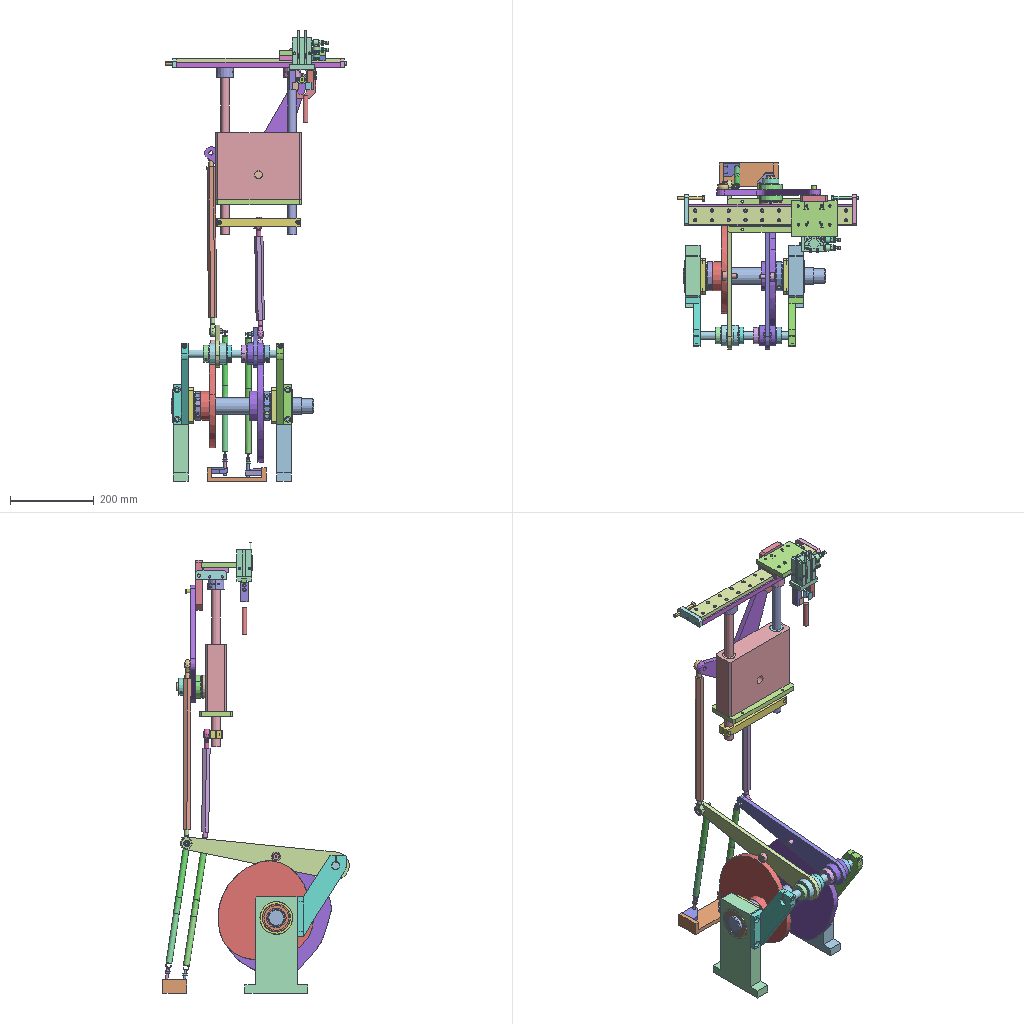Assembly | NX | 112 different items | 112 placed | box 434 x 445 x 1076 mm
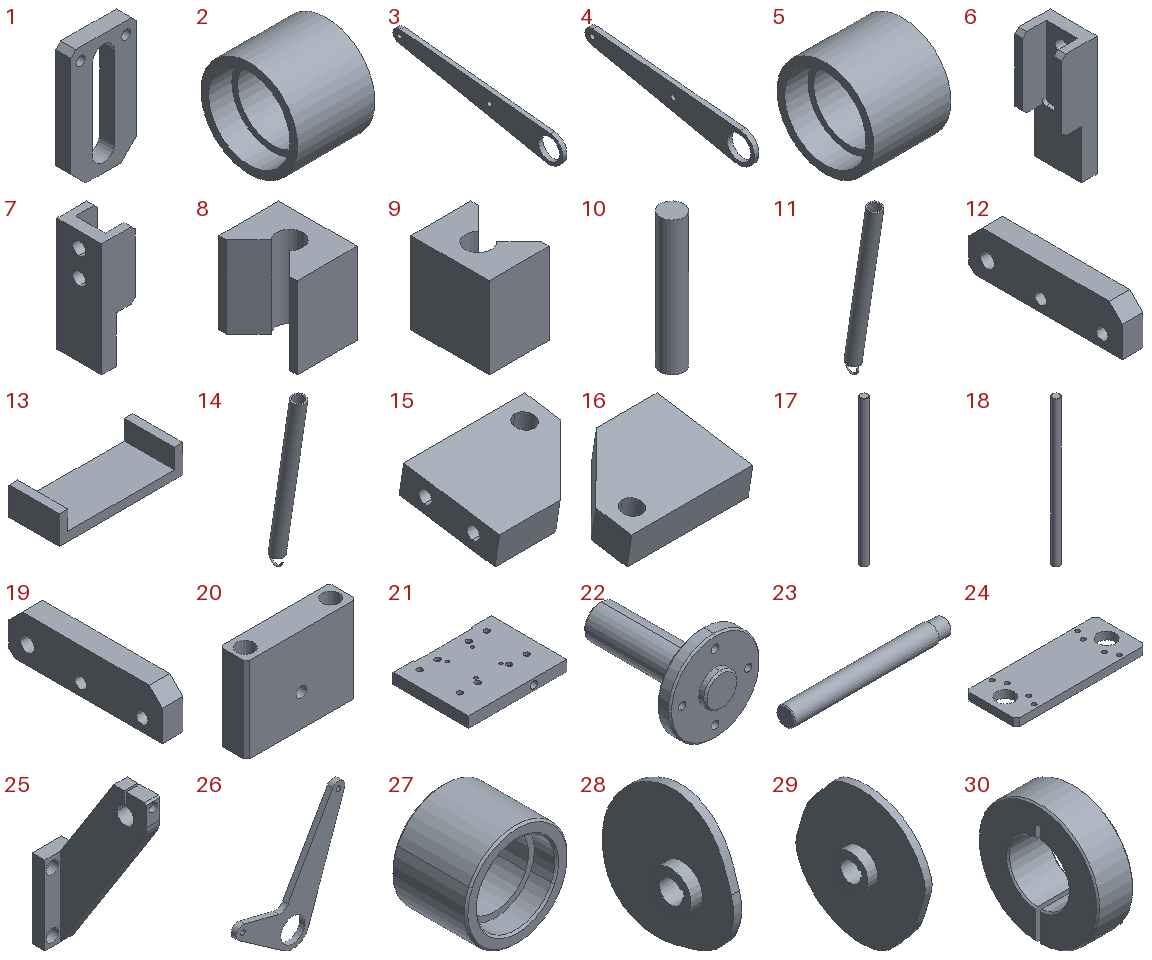Parts list (item | quantity | size | volume | features):
1 | x1 | 65 x 15 x 120 mm | 77204 mm3 | features 001 2
2 | x1 | 40 x 50 x 50 mm | 29003 mm3 | features _-17204000 2
3 | x1 | 10 x 403.429 x 100.813 mm | 170075 mm3 | features _-17232000 2
4 | x1 | 10 x 359.893 x 95.107 mm | 149250 mm3 | features _-17372000 2
5 | x1 | 40 x 50 x 50 mm | 29003 mm3 | features _-17667000 2
6 | x1 | 13.5 x 18 x 45.75 mm | 5474 mm3 | features 倒角2 2
7 | x1 | 13.5 x 18 x 45.75 mm | 5474 mm3 | features 倒角2 2
8 | x1 | 13.775 x 18 x 18.75 mm | 3258 mm3 | features solid 2
9 | x1 | 13.775 x 18 x 18.75 mm | 3258 mm3 | features solid 2
10 | x1 | 11 x 11 x 63 mm | 5987 mm3 | features solid 2
11 | x1 | 14 x 38.697 x 170.602 mm | 9414 mm3 | features solid 2
12 | x1 | 10 x 75 x 21.5 mm | 14819 mm3 | features 001 2
13 | x1 | 141.082 x 56.961 x 32.177 mm | 105625 mm3 | features solid 2
14 | x1 | 14 x 38.402 x 171.464 mm | 9463 mm3 | features solid 2
15 | x1 | 40 x 33.128 x 14.63 mm | 10189 mm3 | features 实体1 2
16 | x1 | 40 x 33.141 x 14.707 mm | 10189 mm3 | features 实体1 2
17 | x1 | 20 x 20 x 400 mm | 125603 mm3 | features 001 2
18 | x1 | 20 x 20 x 400 mm | 125603 mm3 | features 001 2
19 | x1 | 10 x 75 x 21.5 mm | 14819 mm3 | features 001 2
20 | x1 | 205 x 50 x 160 mm | 1357581 mm3 | features 001 2
21 | x1 | 110 x 85 x 12 mm | 106361 mm3 | features 00 2
22 | x1 | 55 x 74 x 55 mm | 38722 mm3 | features 00 2
23 | x1 | 340 x 40 x 40 mm | 417966 mm3 | features 00 2
24 | x1 | 205 x 80 x 12 mm | 176533 mm3 | features 00 2
25 | x1 | 35 x 116.8 x 193.095 mm | 171641 mm3 | features 0004 2
26 | x1 | 247.496 x 12 x 279.945 mm | 214925 mm3 | features 0 2
27 | x1 | 55 x 40 x 55 mm | 45192 mm3 | features 0 2
28 | x1 | 34 x 228.009 x 236.372 mm | 622668 mm3 | features 100X000 2
29 | x1 | 34 x 262.59 x 269.999 mm | 781015 mm3 | features 146X000 2
30 | x1 | 14 x 40 x 39.986 mm | 10434 mm3 | features 1_11 2
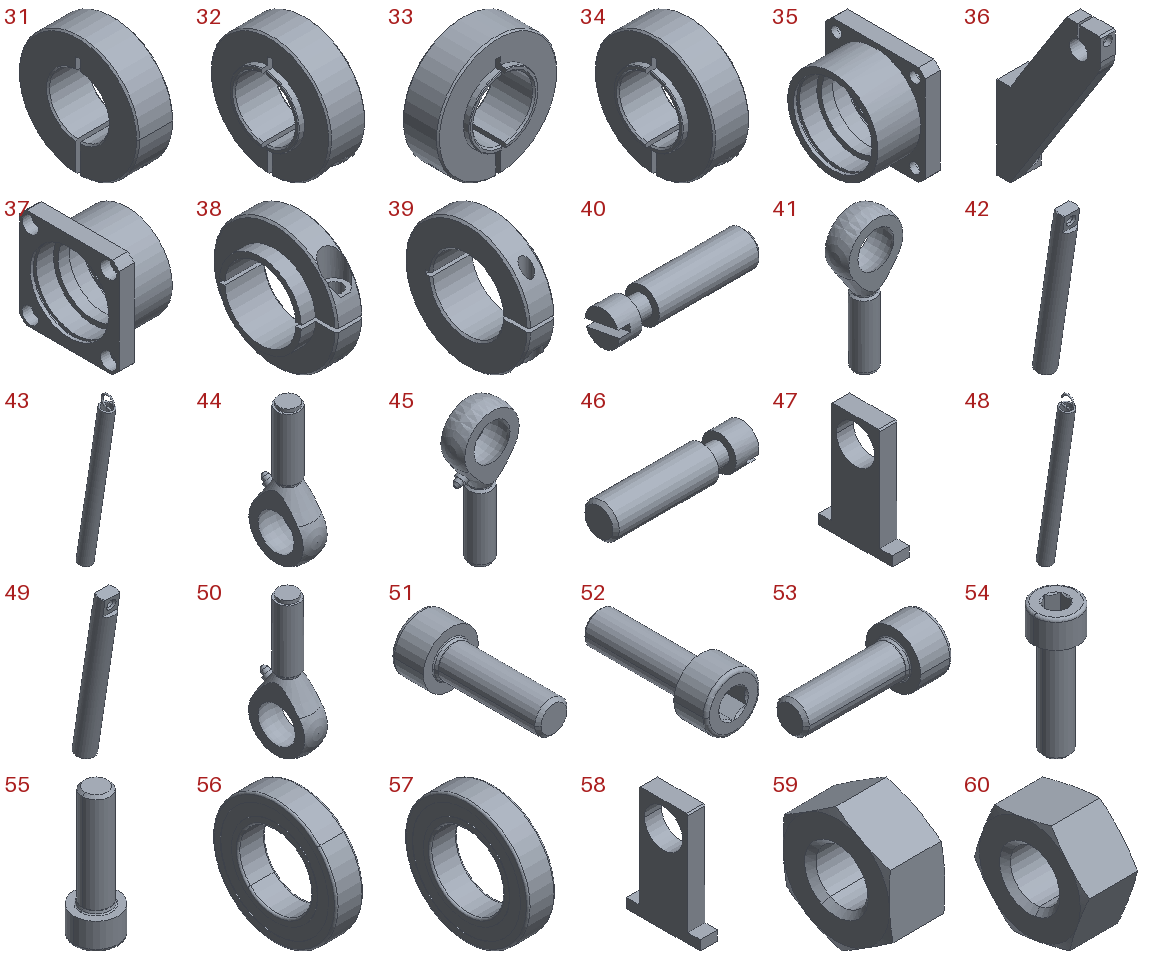31 | x1 | 14 x 40 x 39.986 mm | 10434 mm3 | features 1_11 2
32 | x1 | 14 x 40 x 39.986 mm | 10434 mm3 | features 1_11 2
33 | x1 | 40 x 14 x 39.986 mm | 10434 mm3 | features 1_11 2
34 | x1 | 14 x 40 x 39.986 mm | 10434 mm3 | features 1_11 2
35 | x1 | 50 x 86 x 86 mm | 89594 mm3 | features 1_1 2
36 | x1 | 35 x 116.8 x 193.095 mm | 171641 mm3 | features 0005 2
37 | x1 | 50 x 86 x 86 mm | 89594 mm3 | features 1_1 2
38 | x1 | 23 x 69.986 x 70 mm | 38156 mm3 | features 1_52 2
39 | x1 | 23 x 69.986 x 70 mm | 38156 mm3 | features 1_52 2
40 | x1 | 25 x 6 x 6 mm | 635.671 mm3 | features 1 2
41 | x1 | 26 x 10.639 x 61.044 mm | 5586 mm3 | features 1 2
42 | x1 | 6 x 12.52 x 50.075 mm | 1355 mm3 | features 1 2
43 | x1 | 14 x 39.013 x 172.675 mm | 9539 mm3 | features 1 2
44 | x1 | 11.237 x 26 x 61.087 mm | 5586 mm3 | features 1 2
45 | x1 | 26 x 11.258 x 61.087 mm | 5586 mm3 | features 1 2
46 | x1 | 25 x 6 x 6 mm | 635.671 mm3 | features 1 2
47 | x1 | 35 x 150 x 230 mm | 672442 mm3 | features 0006 2
48 | x1 | 14 x 38.473 x 171.94 mm | 9491 mm3 | features 1 2
49 | x1 | 6 x 12.629 x 50.067 mm | 1355 mm3 | features 1 2
50 | x1 | 11.496 x 26 x 61.044 mm | 5586 mm3 | features 1 2
51 | x1 | 8.5 x 21 x 8.5 mm | 547.645 mm3 | features 2_11 2
52 | x1 | 8.5 x 21 x 8.5 mm | 547.645 mm3 | features 2_11 2
53 | x1 | 21 x 8.5 x 8.5 mm | 547.645 mm3 | features 2_11 2
54 | x1 | 13 x 13 x 38 mm | 2398 mm3 | features 2_12 2
55 | x1 | 13 x 13 x 38 mm | 2398 mm3 | features 2_12 2
56 | x1 | 15 x 68 x 68 mm | 34781 mm3 | features 2_1 2
57 | x1 | 15 x 68 x 68 mm | 34781 mm3 | features 2_1 2
58 | x1 | 35 x 150 x 230 mm | 672442 mm3 | features 0006 2
59 | x1 | 5.2 x 10.241 x 11.536 mm | 345.697 mm3 | features 2 2
60 | x1 | 5.2 x 11.36 x 10.873 mm | 345.697 mm3 | features 2 2
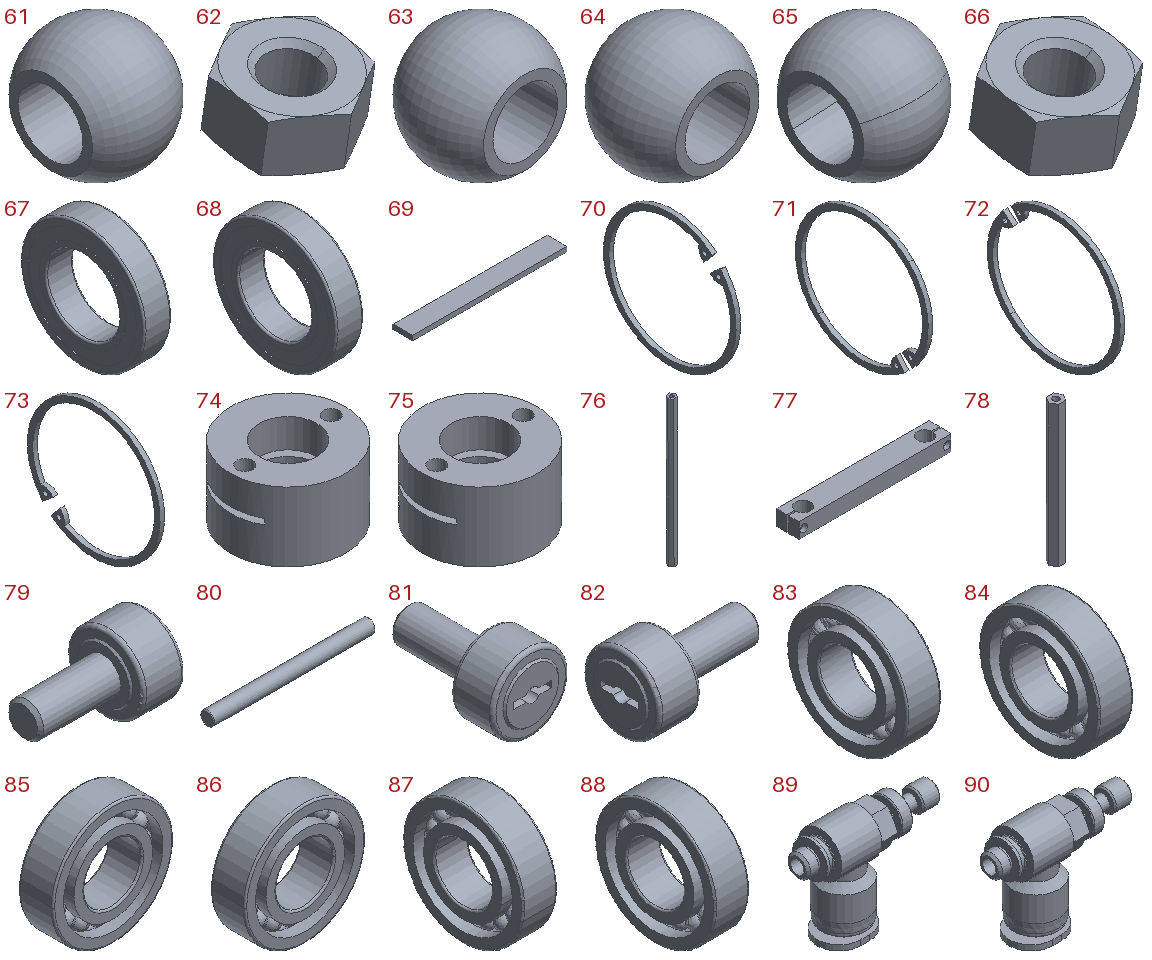61 | x1 | 14.279 x 19.031 x 19.031 mm | 2165 mm3 | features 2 2
62 | x1 | 10.059 x 12.128 x 6.624 mm | 345.697 mm3 | features 2 2
63 | x1 | 19.031 x 14 x 19.031 mm | 2165 mm3 | features 2 2
64 | x1 | 19.031 x 14.284 x 19.031 mm | 2165 mm3 | features 2 2
65 | x1 | - | 2165 mm3 | features 2 2
66 | x1 | 10.059 x 12.136 x 6.647 mm | 345.697 mm3 | features 2 2
67 | x1 | 15 x 68 x 68 mm | 34781 mm3 | features 3 2
68 | x1 | 15 x 68 x 68 mm | 34781 mm3 | features 3 2
69 | x1 | 390 x 50 x 12 mm | 234000 mm3 | features 0008 2
70 | x1 | 2.5 x 72.5 x 72.5 mm | 1667 mm3 | features 4 2
71 | x1 | 2.5 x 72.5 x 72.5 mm | 1667 mm3 | features 4 2
72 | x1 | 2.5 x 72.5 x 72.5 mm | 1667 mm3 | features 5 2
73 | x1 | 2.5 x 72.5 x 72.5 mm | 1667 mm3 | features 5 2
74 | x1 | 40 x 40 x 24 mm | 19127 mm3 | features A0001 2
75 | x1 | 40 x 40 x 24 mm | 19127 mm3 | features A0001 2
76 | x1 | 23.181 x 19.188 x 360.176 mm | 87224 mm3 | features A0 2
77 | x1 | 200 x 30 x 20 mm | 103319 mm3 | features B0002 2
78 | x1 | 23.011 x 20.454 x 200.401 mm | 47179 mm3 | features B0 2
79 | x1 | 36 x 22 x 22 mm | 6364 mm3 | features CFFRC10-22 2
80 | x1 | 236 x 20 x 20 mm | 74081 mm3 | features 000 2
81 | x1 | 22 x 36 x 22 mm | 6364 mm3 | features CFFRC10-22 2
82 | x1 | 36 x 22 x 22 mm | 6364 mm3 | features CFFRC10-22 2
83 | x1 | 12 x 42 x 42 mm | 9438 mm3 | features DEEP_GROOVE_BALL_BEARINGS_GB_RO 2
84 | x1 | 12 x 42 x 42 mm | 9438 mm3 | features DEEP_GROOVE_BALL_BEARINGS_GB_RO 2
85 | x1 | 42 x 12 x 42 mm | 9438 mm3 | features DEEP_GROOVE_BALL_BEARINGS_GB_RO 2
86 | x1 | 42 x 12 x 42 mm | 9438 mm3 | features DEEP_GROOVE_BALL_BEARINGS_GB_RO 2
87 | x1 | 12 x 42 x 42 mm | 9438 mm3 | features DEEP_GROOVE_BALL_BEARINGS_GB_RO 2
88 | x1 | 12 x 42 x 42 mm | 9438 mm3 | features DEEP_GROOVE_BALL_BEARINGS_GB_RO 2
89 | x1 | 44.567 x 15.75 x 33.6 mm | 6449 mm3 | features J-XZB01-D6-M5.SLDPRT 2
90 | x1 | 44.567 x 15.75 x 33.6 mm | 6449 mm3 | features J-XZB01-D6-M5.SLDPRT 2
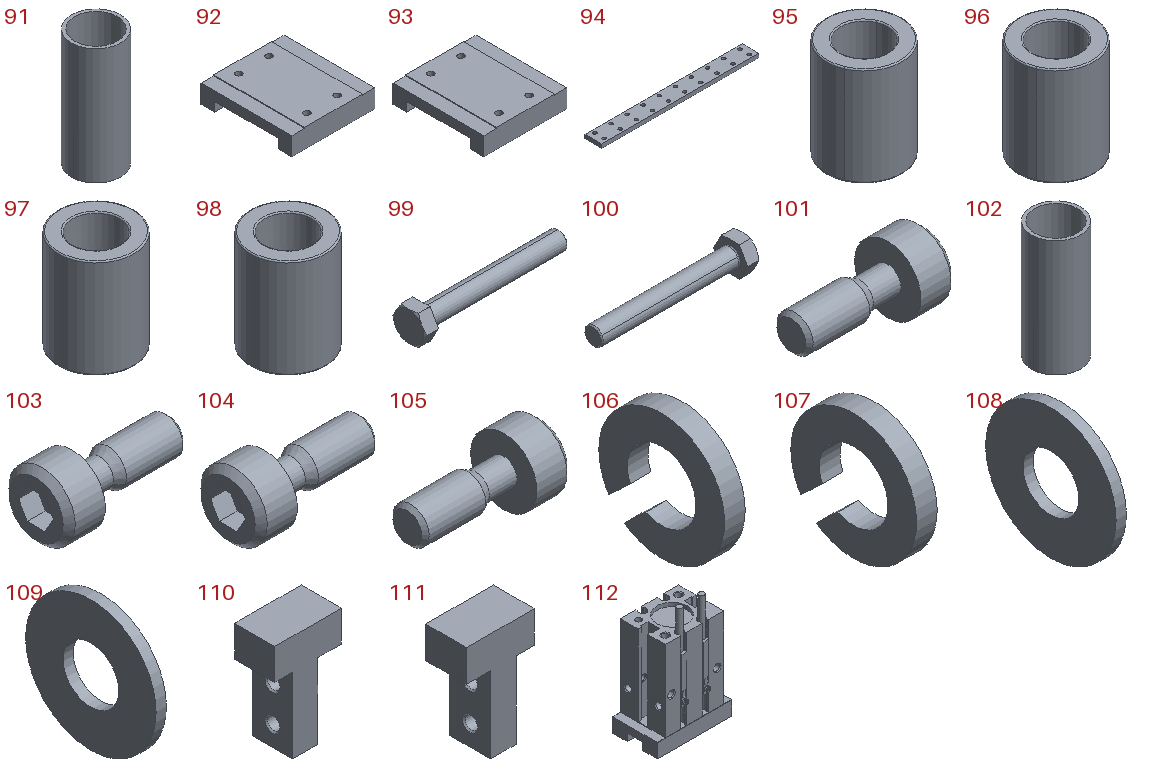91 | x1 | 32 x 32 x 76 mm | 14326 mm3 | features 0018 2
92 | x1 | 54.8 x 60 x 12.6 mm | 26674 mm3 | features MGW_MGN15C00 2
93 | x1 | 54.8 x 60 x 12.6 mm | 26674 mm3 | features MGW_MGN15C00 2
94 | x1 | 390 x 42 x 9.5 mm | 149496 mm3 | features MGW_MGWR15R3900001 2
95 | x1 | 32 x 32 x 42 mm | 20566 mm3 | features MISUMI__LMU-N200001 2
96 | x1 | 32 x 32 x 42 mm | 20566 mm3 | features MISUMI__LMU-N200001 2
97 | x1 | 32 x 32 x 42 mm | 20566 mm3 | features MISUMI__LMU-N200001 2
98 | x1 | 32 x 32 x 42 mm | 20566 mm3 | features MISUMI__LMU-N200001 2
99 | x1 | 65.5 x 15 x 13 mm | 3817 mm3 | features STRCB8-60 2
100 | x1 | 65.5 x 15 x 13 mm | 3817 mm3 | features STRCB8-60 2
101 | x1 | 16.5 x 8.25 x 8.25 mm | 366.306 mm3 | features TAM02-M3-L8-001 2
102 | x1 | 32 x 32 x 76 mm | 14326 mm3 | features 0018 2
103 | x1 | 16.5 x 8.25 x 8.25 mm | 366.306 mm3 | features TAM02-M3-L8-001 2
104 | x1 | 16.5 x 8.25 x 8.25 mm | 366.306 mm3 | features TAM02-M3-L8-001 2
105 | x1 | 16.5 x 8.25 x 8.25 mm | 366.306 mm3 | features TAM02-M3-L8-001 2
106 | x1 | 1.35 x 8.25 x 8.25 mm | 46.859 mm3 | features TAM02-M3-L8-002 2
107 | x1 | 1.35 x 8.25 x 8.25 mm | 46.859 mm3 | features TAM02-M3-L8-002 2
108 | x1 | 0.825 x 10.5 x 10.5 mm | 58.316 mm3 | features TAM02-M3-L8-003 2
109 | x1 | 0.825 x 10.5 x 10.5 mm | 58.316 mm3 | features TAM02-M3-L8-003 2
110 | x1 | 19.85 x 12 x 31.8 mm | 4076 mm3 | features WGY01-16-6-2-001 2
111 | x1 | 19.85 x 12 x 31.8 mm | 4076 mm3 | features WGY01-16-6-2-001 2
112 | x1 | 58.5 x 37.65 x 92.25 mm | 104769 mm3 | features WGY01-16-6-2-002 2